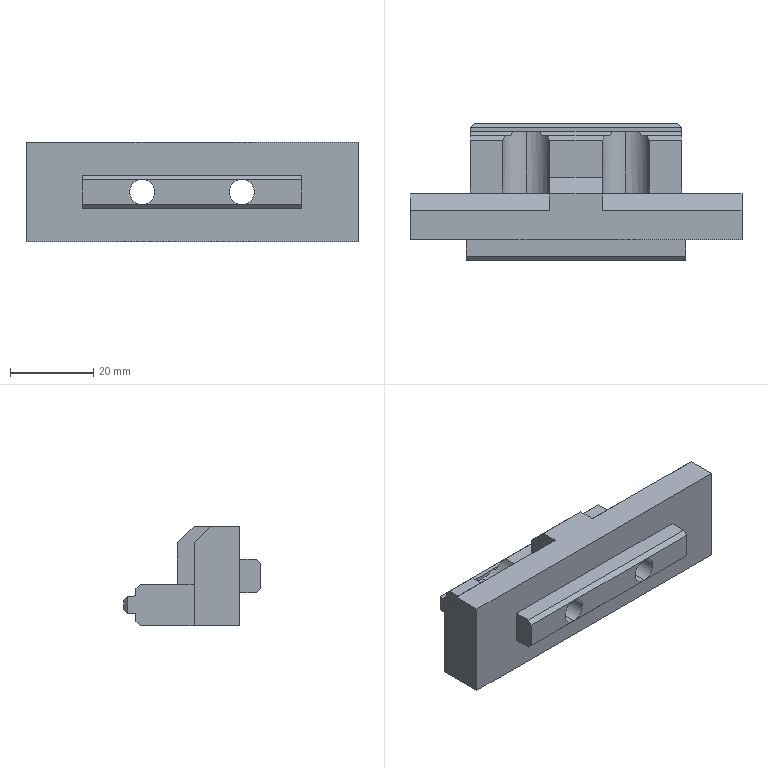Part | SolidWorks | features ICE 7, Chamfer 3, Extrusion 1, Fillet 1 | 1 solid | 61 faces | box 80 x 33 x 24 mm | volume 28866 mm3 | plane 46 | cylinder 15 | commonest cylinder face diameters 6 x4 8 x4 12 x4 2 x3